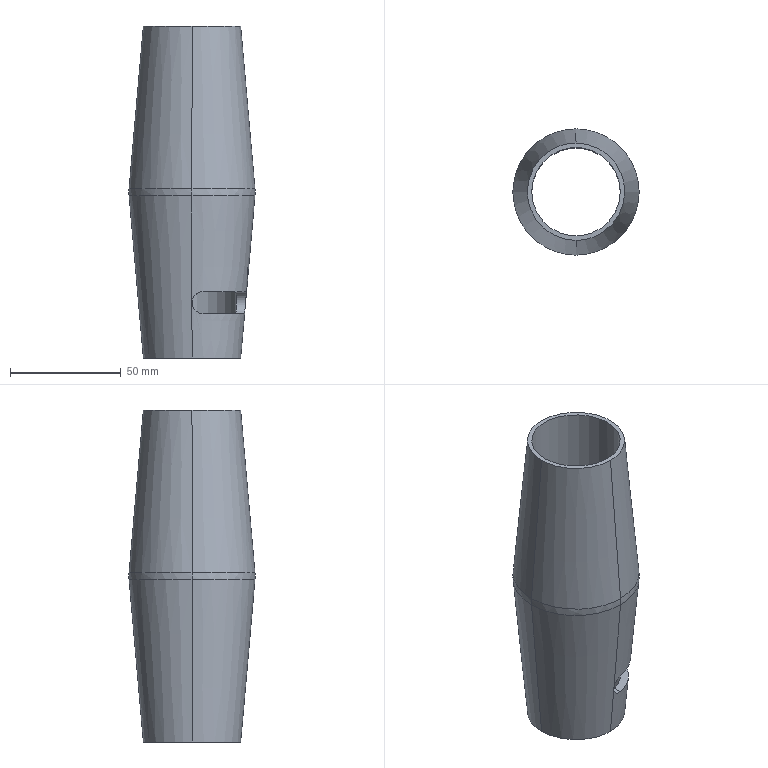Part | NX | features EXTRACT_STRING 12, THRU_CURVE_MESH 8, DATUM_CSYS 6, SKETCH 5, LINE 4, Instance Feature 3, Mirror Feature 3, DATUM_PLANE 2, EXTRACT_DATUM_AXIS 2, EXTRACT_DATUM_PLANE 2, EXTRUDE 2, FILL_HOLE 2, BLEND 1, FACE_BLEND 1, SEW 1 | 1 solid | 20 faces | box 57.039 x 57.039 x 150 mm | volume 113335 mm3 | spline 13 | plane 4 | cylinder 3 | commonest cylinder face diameters 10 x2 40 x1
STEP:
#1=CARTESIAN_POINT('',(28.442,0.000000001,76.752));
#2=VERTEX_POINT('',#1);
#3=CARTESIAN_POINT('',(28.442,0.000000001,73.248));
#4=VERTEX_POINT('',#3);
#5=CARTESIAN_POINT('',(8.519,0.000000001,75.));
#6=DIRECTION('',(0.,1.,0.));
#7=DIRECTION('',(0.,0.,1.));
#8=AXIS2_PLACEMENT_3D('',#5,#6,#7);
#9=CIRCLE('',#8,20.);
#10=EDGE_CURVE('',#2,#4,#9,.T.);
#11=ORIENTED_EDGE('',*,*,#10,.F.);
#12=CARTESIAN_POINT('',(0.,-28.442,76.752));
#13=VERTEX_POINT('',#12);
#14=CARTESIAN_POINT('',(0.,-28.442,76.752));
#15=CARTESIAN_POINT('',(3.703,-28.442,76.752));
#16=CARTESIAN_POINT('',(11.179,-26.96,76.752));
#17=CARTESIAN_POINT('',(20.625,-20.641,76.752));
#18=CARTESIAN_POINT('',(26.948,-11.192,76.752));
#19=CARTESIAN_POINT('',(28.442,-3.756,76.752));
#20=CARTESIAN_POINT('',(28.442,0.000000001,76.752));
#21=B_SPLINE_CURVE_WITH_KNOTS('',3,(#14,#15,#16,#17,#18,#19,#20),.UNSPECIFIED.,.F.,.F.,(4,1,1,1,4),(-0.00000006,0.01111,0.02222,0.03332,0.04443),.UNSPECIFIED.);
#22=EDGE_CURVE('',#13,#2,#21,.T.);
#23=ORIENTED_EDGE('',*,*,#22,.F.);
#24=CARTESIAN_POINT('',(0.,-28.442,73.248));
#25=VERTEX_POINT('',#24);
#26=CARTESIAN_POINT('',(0.,-8.519,75.));
#27=DIRECTION('',(1.,0.,0.));
#28=DIRECTION('',(0.,1.,0.));
#29=AXIS2_PLACEMENT_3D('',#26,#27,#28);
#30=CIRCLE('',#29,20.);
#31=EDGE_CURVE('',#13,#25,#30,.T.);
#32=ORIENTED_EDGE('',*,*,#31,.T.);
#33=CARTESIAN_POINT('',(28.442,0.000000001,73.248));
#34=CARTESIAN_POINT('',(28.442,-3.733,73.248));
#35=CARTESIAN_POINT('',(26.948,-11.202,73.248));
#36=CARTESIAN_POINT('',(20.623,-20.639,73.248));
#37=CARTESIAN_POINT('',(12.759,-25.903,73.248));
#38=CARTESIAN_POINT('',(5.563,-28.078,73.248));
#39=CARTESIAN_POINT('',(1.878,-28.442,73.248));
#40=CARTESIAN_POINT('',(0.,-28.442,73.248));
#41=B_SPLINE_CURVE_WITH_KNOTS('',3,(#33,#34,#35,#36,#37,#38,#39,#40),.UNSPECIFIED.,.F.,.F.,(4,1,1,1,1,4),(-0.00000006,0.0112,0.0224,0.0336,0.03919,0.04479),.UNSPECIFIED.);
#42=EDGE_CURVE('',#4,#25,#41,.T.);
#43=ORIENTED_EDGE('',*,*,#42,.F.);
#44=EDGE_LOOP('',(#11,#23,#32,#43));
#45=FACE_BOUND('',#44,.T.);
#46=CARTESIAN_POINT('',(0.000000001,-28.442,73.248));
#47=CARTESIAN_POINT('',(0.,-28.597,75.));
#48=CARTESIAN_POINT('',(0.,-28.442,76.752));
#49=CARTESIAN_POINT('',(1.895,-28.442,73.248));
#50=CARTESIAN_POINT('',(1.905,-28.597,75.));
#51=CARTESIAN_POINT('',(1.895,-28.442,76.752));
#52=CARTESIAN_POINT('',(5.564,-28.077,73.248));
#53=CARTESIAN_POINT('',(5.594,-28.229,75.));
#54=CARTESIAN_POINT('',(5.564,-28.077,76.752));
#55=CARTESIAN_POINT('',(12.78,-25.896,73.248));
#56=CARTESIAN_POINT('',(12.849,-26.037,75.));
#57=CARTESIAN_POINT('',(12.78,-25.896,76.752));
#58=CARTESIAN_POINT('',(20.647,-20.616,73.248));
#59=CARTESIAN_POINT('',(20.759,-20.728,75.));
#60=CARTESIAN_POINT('',(20.647,-20.616,76.752));
#61=CARTESIAN_POINT('',(25.914,-12.739,73.248));
#62=CARTESIAN_POINT('',(26.054,-12.808,75.));
#63=CARTESIAN_POINT('',(25.914,-12.739,76.752));
#64=CARTESIAN_POINT('',(28.083,-5.538,73.248));
#65=CARTESIAN_POINT('',(28.236,-5.568,75.));
#66=CARTESIAN_POINT('',(28.083,-5.538,76.752));
#67=CARTESIAN_POINT('',(28.442,-1.857,73.248));
#68=CARTESIAN_POINT('',(28.597,-1.867,75.));
#69=CARTESIAN_POINT('',(28.442,-1.857,76.752));
#70=CARTESIAN_POINT('',(28.442,0.000000001,73.248));
#71=CARTESIAN_POINT('',(28.597,0.000000001,75.));
#72=CARTESIAN_POINT('',(28.442,0.000000001,76.752));
#73=(BOUNDED_SURFACE()B_SPLINE_SURFACE(3,2,((#46,#47,#48),(#49,#50,#51),(#52,#53,#54),(#55,#56,#57),(#58,#59,#60),(#61,#62,#63),(#64,#65,#66),(#67,#68,#69),(#70,#71,#72)),.UNSPECIFIED.,.F.,.F.,.F.)B_SPLINE_SURFACE_WITH_KNOTS((4,1,1,1,1,1,4),(3,3),(0.07773,0.07942,0.08111,0.08449,0.08787,0.08956,0.09125),(0.,1.),.UNSPECIFIED.)GEOMETRIC_REPRESENTATION_ITEM()RATIONAL_B_SPLINE_SURFACE(((1.,0.9962,1.),(1.,0.9962,1.),(1.,0.9962,1.),(1.,0.9962,1.),(1.,0.9962,1.),(1.,0.9962,1.),(1.,0.9962,1.),(1.,0.9962,1.),(1.,0.9962,1.)))REPRESENTATION_ITEM('')SURFACE());
#74=ADVANCED_FACE('',(#45),#73,.T.);
#75=ORIENTED_EDGE('',*,*,#31,.F.);
#76=CARTESIAN_POINT('',(-28.442,-0.000000001,76.752));
#77=VERTEX_POINT('',#76);
#78=CARTESIAN_POINT('',(-28.442,0.,76.752));
#79=CARTESIAN_POINT('',(-28.442,-3.733,76.752));
#80=CARTESIAN_POINT('',(-26.948,-11.202,76.752));
#81=CARTESIAN_POINT('',(-20.623,-20.639,76.752));
#82=CARTESIAN_POINT('',(-12.759,-25.903,76.752));
#83=CARTESIAN_POINT('',(-5.563,-28.078,76.752));
#84=CARTESIAN_POINT('',(-1.878,-28.442,76.752));
#85=CARTESIAN_POINT('',(0.,-28.442,76.752));
#86=B_SPLINE_CURVE_WITH_KNOTS('',3,(#78,#79,#80,#81,#82,#83,#84,#85),.UNSPECIFIED.,.F.,.F.,(4,1,1,1,1,4),(-0.00000006,0.0112,0.0224,0.0336,0.03919,0.04479),.UNSPECIFIED.);
#87=EDGE_CURVE('',#77,#13,#86,.T.);
#88=ORIENTED_EDGE('',*,*,#87,.F.);
#89=CARTESIAN_POINT('',(-28.442,0.,73.248));
#90=VERTEX_POINT('',#89);
#91=CARTESIAN_POINT('',(-8.519,0.,75.));
#92=DIRECTION('',(0.,-1.,0.));
#93=DIRECTION('',(0.,0.,-1.));
#94=AXIS2_PLACEMENT_3D('',#91,#92,#93);
#95=CIRCLE('',#94,20.);
#96=EDGE_CURVE('',#77,#90,#95,.T.);
#97=ORIENTED_EDGE('',*,*,#96,.T.);
#98=CARTESIAN_POINT('',(0.,-28.442,73.248));
#99=CARTESIAN_POINT('',(-3.703,-28.442,73.248));
#100=CARTESIAN_POINT('',(-11.179,-26.96,73.248));
#101=CARTESIAN_POINT('',(-20.625,-20.641,73.248));
#102=CARTESIAN_POINT('',(-26.948,-11.192,73.248));
#103=CARTESIAN_POINT('',(-28.442,-3.756,73.248));
#104=CARTESIAN_POINT('',(-28.442,0.,73.248));
#105=B_SPLINE_CURVE_WITH_KNOTS('',3,(#98,#99,#100,#101,#102,#103,#104),.UNSPECIFIED.,.F.,.F.,(4,1,1,1,4),(-0.00000006,0.01111,0.02222,0.03332,0.04443),.UNSPECIFIED.);
#106=EDGE_CURVE('',#25,#90,#105,.T.);
#107=ORIENTED_EDGE('',*,*,#106,.F.);
#108=EDGE_LOOP('',(#75,#88,#97,#107));
#109=FACE_BOUND('',#108,.T.);
#110=CARTESIAN_POINT('',(0.,-28.442,76.752));
#111=CARTESIAN_POINT('',(0.,-28.597,75.));
#112=CARTESIAN_POINT('',(0.,-28.442,73.248));
#113=CARTESIAN_POINT('',(-1.895,-28.442,76.752));
#114=CARTESIAN_POINT('',(-1.905,-28.597,75.));
#115=CARTESIAN_POINT('',(-1.895,-28.442,73.248));
#116=CARTESIAN_POINT('',(-5.564,-28.077,76.752));
#117=CARTESIAN_POINT('',(-5.594,-28.229,75.));
#118=CARTESIAN_POINT('',(-5.564,-28.077,73.248));
#119=CARTESIAN_POINT('',(-12.78,-25.896,76.752));
#120=CARTESIAN_POINT('',(-12.849,-26.037,75.));
#121=CARTESIAN_POINT('',(-12.78,-25.896,73.248));
#122=CARTESIAN_POINT('',(-20.647,-20.616,76.752));
#123=CARTESIAN_POINT('',(-20.759,-20.728,75.));
#124=CARTESIAN_POINT('',(-20.647,-20.616,73.248));
#125=CARTESIAN_POINT('',(-25.914,-12.739,76.752));
#126=CARTESIAN_POINT('',(-26.054,-12.808,75.));
#127=CARTESIAN_POINT('',(-25.914,-12.739,73.248));
#128=CARTESIAN_POINT('',(-28.083,-5.538,76.752));
#129=CARTESIAN_POINT('',(-28.236,-5.568,75.));
#130=CARTESIAN_POINT('',(-28.083,-5.538,73.248));
#131=CARTESIAN_POINT('',(-28.442,-1.857,76.752));
#132=CARTESIAN_POINT('',(-28.597,-1.867,75.));
#133=CARTESIAN_POINT('',(-28.442,-1.857,73.248));
#134=CARTESIAN_POINT('',(-28.442,0.,76.752));
#135=CARTESIAN_POINT('',(-28.597,0.,75.));
#136=CARTESIAN_POINT('',(-28.442,0.,73.248));
#137=(BOUNDED_SURFACE()B_SPLINE_SURFACE(3,2,((#110,#111,#112),(#113,#114,#115),(#116,#117,#118),(#119,#120,#121),(#122,#123,#124),(#125,#126,#127),(#128,#129,#130),(#131,#132,#133),(#134,#135,#136)),.UNSPECIFIED.,.F.,.F.,.F.)B_SPLINE_SURFACE_WITH_KNOTS((4,1,1,1,1,1,4),(3,3),(0.,0.001666,0.003332,0.006664,0.009996,0.01166,0.01333),(0.,1.),.UNSPECIFIED.)GEOMETRIC_REPRESENTATION_ITEM()RATIONAL_B_SPLINE_SURFACE(((1.,0.9962,1.),(1.,0.9962,1.),(1.,0.9962,1.),(1.,0.9962,1.),(1.,0.9962,1.),(1.,0.9962,1.),(1.,0.9962,1.),(1.,0.9962,1.),(1.,0.9962,1.)))REPRESENTATION_ITEM('')SURFACE());
#138=ADVANCED_FACE('',(#109),#137,.T.);
#139=ORIENTED_EDGE('',*,*,#96,.F.);
#140=CARTESIAN_POINT('',(-0.000000001,28.442,76.752));
#141=VERTEX_POINT('',#140);
#142=CARTESIAN_POINT('',(-0.000000001,28.442,76.752));
#143=CARTESIAN_POINT('',(-3.733,28.442,76.752));
#144=CARTESIAN_POINT('',(-11.202,26.948,76.752));
#145=CARTESIAN_POINT('',(-20.639,20.623,76.752));
#146=CARTESIAN_POINT('',(-25.903,12.759,76.752));
#147=CARTESIAN_POINT('',(-28.078,5.563,76.752));
#148=CARTESIAN_POINT('',(-28.442,1.878,76.752));
#149=CARTESIAN_POINT('',(-28.442,-0.000000001,76.752));
#150=B_SPLINE_CURVE_WITH_KNOTS('',3,(#142,#143,#144,#145,#146,#147,#148,#149),.UNSPECIFIED.,.F.,.F.,(4,1,1,1,1,4),(-0.00000006,0.0112,0.0224,0.0336,0.03919,0.04479),.UNSPECIFIED.);
#151=EDGE_CURVE('',#141,#77,#150,.T.);
#152=ORIENTED_EDGE('',*,*,#151,.F.);
#153=CARTESIAN_POINT('',(0.,28.442,73.248));
#154=VERTEX_POINT('',#153);
#155=CARTESIAN_POINT('',(0.,8.519,75.));
#156=DIRECTION('',(-1.,0.,0.));
#157=DIRECTION('',(0.,0.,1.));
#158=AXIS2_PLACEMENT_3D('',#155,#156,#157);
#159=CIRCLE('',#158,20.);
#160=EDGE_CURVE('',#141,#154,#159,.T.);
#161=ORIENTED_EDGE('',*,*,#160,.T.);
#162=CARTESIAN_POINT('',(-28.442,0.,73.248));
#163=CARTESIAN_POINT('',(-28.442,3.703,73.248));
#164=CARTESIAN_POINT('',(-26.96,11.179,73.248));
#165=CARTESIAN_POINT('',(-20.641,20.625,73.248));
#166=CARTESIAN_POINT('',(-11.192,26.948,73.248));
#167=CARTESIAN_POINT('',(-3.756,28.442,73.248));
#168=CARTESIAN_POINT('',(0.,28.442,73.248));
#169=B_SPLINE_CURVE_WITH_KNOTS('',3,(#162,#163,#164,#165,#166,#167,#168),.UNSPECIFIED.,.F.,.F.,(4,1,1,1,4),(-0.00000006,0.01111,0.02222,0.03332,0.04443),.UNSPECIFIED.);
#170=EDGE_CURVE('',#90,#154,#169,.T.);
#171=ORIENTED_EDGE('',*,*,#170,.F.);
#172=EDGE_LOOP('',(#139,#152,#161,#171));
#173=FACE_BOUND('',#172,.T.);
#174=CARTESIAN_POINT('',(-28.442,-0.000000001,76.752));
#175=CARTESIAN_POINT('',(-28.597,0.,75.));
#176=CARTESIAN_POINT('',(-28.442,0.,73.248));
#177=CARTESIAN_POINT('',(-28.442,1.895,76.752));
#178=CARTESIAN_POINT('',(-28.597,1.905,75.));
#179=CARTESIAN_POINT('',(-28.442,1.895,73.248));
#180=CARTESIAN_POINT('',(-28.077,5.564,76.752));
#181=CARTESIAN_POINT('',(-28.229,5.594,75.));
#182=CARTESIAN_POINT('',(-28.077,5.564,73.248));
#183=CARTESIAN_POINT('',(-25.896,12.78,76.752));
#184=CARTESIAN_POINT('',(-26.037,12.849,75.));
#185=CARTESIAN_POINT('',(-25.896,12.78,73.248));
#186=CARTESIAN_POINT('',(-20.616,20.647,76.752));
#187=CARTESIAN_POINT('',(-20.728,20.759,75.));
#188=CARTESIAN_POINT('',(-20.616,20.647,73.248));
#189=CARTESIAN_POINT('',(-12.739,25.914,76.752));
#190=CARTESIAN_POINT('',(-12.808,26.054,75.));
#191=CARTESIAN_POINT('',(-12.739,25.914,73.248));
#192=CARTESIAN_POINT('',(-5.538,28.083,76.752));
#193=CARTESIAN_POINT('',(-5.568,28.236,75.));
#194=CARTESIAN_POINT('',(-5.538,28.083,73.248));
#195=CARTESIAN_POINT('',(-1.857,28.442,76.752));
#196=CARTESIAN_POINT('',(-1.867,28.597,75.));
#197=CARTESIAN_POINT('',(-1.857,28.442,73.248));
#198=CARTESIAN_POINT('',(-0.000000001,28.442,76.752));
#199=CARTESIAN_POINT('',(0.,28.597,75.));
#200=CARTESIAN_POINT('',(0.,28.442,73.248));
#201=(BOUNDED_SURFACE()B_SPLINE_SURFACE(3,2,((#174,#175,#176),(#177,#178,#179),(#180,#181,#182),(#183,#184,#185),(#186,#187,#188),(#189,#190,#191),(#192,#193,#194),(#195,#196,#197),(#198,#199,#200)),.UNSPECIFIED.,.F.,.F.,.F.)B_SPLINE_SURFACE_WITH_KNOTS((4,1,1,1,1,1,4),(3,3),(0.,0.001666,0.003332,0.006664,0.009996,0.01166,0.01333),(0.,1.),.UNSPECIFIED.)GEOMETRIC_REPRESENTATION_ITEM()RATIONAL_B_SPLINE_SURFACE(((1.,0.9962,1.),(1.,0.9962,1.),(1.,0.9962,1.),(1.,0.9962,1.),(1.,0.9962,1.),(1.,0.9962,1.),(1.,0.9962,1.),(1.,0.9962,1.),(1.,0.9962,1.)))REPRESENTATION_ITEM('')SURFACE());
#202=ADVANCED_FACE('',(#173),#201,.T.);
#203=CARTESIAN_POINT('',(28.442,0.000000001,76.752));
#204=CARTESIAN_POINT('',(28.442,3.733,76.752));
#205=CARTESIAN_POINT('',(26.948,11.202,76.752));
#206=CARTESIAN_POINT('',(20.623,20.639,76.752));
#207=CARTESIAN_POINT('',(12.759,25.903,76.752));
#208=CARTESIAN_POINT('',(5.563,28.078,76.752));
#209=CARTESIAN_POINT('',(1.878,28.442,76.752));
#210=CARTESIAN_POINT('',(-0.000000001,28.442,76.752));
#211=B_SPLINE_CURVE_WITH_KNOTS('',3,(#203,#204,#205,#206,#207,#208,#209,#210),.UNSPECIFIED.,.F.,.F.,(4,1,1,1,1,4),(-0.00000006,0.0112,0.0224,0.0336,0.03919,0.04479),.UNSPECIFIED.);
#212=EDGE_CURVE('',#2,#141,#211,.T.);
#213=ORIENTED_EDGE('',*,*,#212,.F.);
#214=ORIENTED_EDGE('',*,*,#10,.T.);
#215=CARTESIAN_POINT('',(-0.000000001,28.442,73.248));
#216=CARTESIAN_POINT('',(3.703,28.442,73.248));
#217=CARTESIAN_POINT('',(11.179,26.96,73.248));
#218=CARTESIAN_POINT('',(20.625,20.641,73.248));
#219=CARTESIAN_POINT('',(26.948,11.192,73.248));
#220=CARTESIAN_POINT('',(28.442,3.756,73.248));
#221=CARTESIAN_POINT('',(28.442,0.000000001,73.248));
#222=B_SPLINE_CURVE_WITH_KNOTS('',3,(#215,#216,#217,#218,#219,#220,#221),.UNSPECIFIED.,.F.,.F.,(4,1,1,1,4),(-0.00000006,0.01111,0.02222,0.03332,0.04443),.UNSPECIFIED.);
#223=EDGE_CURVE('',#154,#4,#222,.T.);
#224=ORIENTED_EDGE('',*,*,#223,.F.);
#225=ORIENTED_EDGE('',*,*,#160,.F.);
#226=EDGE_LOOP('',(#213,#214,#224,#225));
#227=FACE_BOUND('',#226,.T.);
#228=CARTESIAN_POINT('',(-0.000000001,28.442,76.752));
#229=CARTESIAN_POINT('',(-0.000000001,28.597,75.));
#230=CARTESIAN_POINT('',(-0.000000001,28.442,73.248));
#231=CARTESIAN_POINT('',(1.895,28.442,76.752));
#232=CARTESIAN_POINT('',(1.905,28.597,75.));
#233=CARTESIAN_POINT('',(1.895,28.442,73.248));
#234=CARTESIAN_POINT('',(5.564,28.077,76.752));
#235=CARTESIAN_POINT('',(5.594,28.229,75.));
#236=CARTESIAN_POINT('',(5.564,28.077,73.248));
#237=CARTESIAN_POINT('',(12.78,25.896,76.752));
#238=CARTESIAN_POINT('',(12.849,26.037,75.));
#239=CARTESIAN_POINT('',(12.78,25.896,73.248));
#240=CARTESIAN_POINT('',(20.647,20.616,76.752));
#241=CARTESIAN_POINT('',(20.759,20.728,75.));
#242=CARTESIAN_POINT('',(20.647,20.616,73.248));
#243=CARTESIAN_POINT('',(25.914,12.739,76.752));
#244=CARTESIAN_POINT('',(26.054,12.808,75.));
#245=CARTESIAN_POINT('',(25.914,12.739,73.248));
#246=CARTESIAN_POINT('',(28.083,5.538,76.752));
#247=CARTESIAN_POINT('',(28.236,5.568,75.));
#248=CARTESIAN_POINT('',(28.083,5.538,73.248));
#249=CARTESIAN_POINT('',(28.442,1.857,76.752));
#250=CARTESIAN_POINT('',(28.597,1.867,75.));
#251=CARTESIAN_POINT('',(28.442,1.857,73.248));
#252=CARTESIAN_POINT('',(28.442,0.000000001,76.752));
#253=CARTESIAN_POINT('',(28.597,0.000000001,75.));
#254=CARTESIAN_POINT('',(28.442,0.000000001,73.248));
#255=(BOUNDED_SURFACE()B_SPLINE_SURFACE(3,2,((#228,#229,#230),(#231,#232,#233),(#234,#235,#236),(#237,#238,#239),(#240,#241,#242),(#243,#244,#245),(#246,#247,#248),(#249,#250,#251),(#252,#253,#254)),.UNSPECIFIED.,.F.,.F.,.F.)B_SPLINE_SURFACE_WITH_KNOTS((4,1,1,1,1,1,4),(3,3),(0.,0.001666,0.003332,0.006664,0.009996,0.01166,0.01333),(0.,1.),.UNSPECIFIED.)GEOMETRIC_REPRESENTATION_ITEM()RATIONAL_B_SPLINE_SURFACE(((1.,0.9962,1.),(1.,0.9962,1.),(1.,0.9962,1.),(1.,0.9962,1.),(1.,0.9962,1.),(1.,0.9962,1.),(1.,0.9962,1.),(1.,0.9962,1.),(1.,0.9962,1.)))REPRESENTATION_ITEM('')SURFACE());
#256=ADVANCED_FACE('',(#227),#255,.T.);
#257=CARTESIAN_POINT('',(24.199,0.,25.));
#258=VERTEX_POINT('',#257);
#259=CARTESIAN_POINT('',(28.597,0.000000001,75.));
#260=CARTESIAN_POINT('',(26.398,0.000000001,50.));
#261=CARTESIAN_POINT('',(24.199,0.,25.));
#262=CARTESIAN_POINT('',(22.,0.,0.));
#263=B_SPLINE_CURVE_WITH_KNOTS('',3,(#259,#260,#261,#262),.UNSPECIFIED.,.F.,.F.,(4,4),(0.,1.),.PIECEWISE_BEZIER_KNOTS.);
#264=EDGE_CURVE('',#258,#4,#263,.F.);
#265=ORIENTED_EDGE('',*,*,#264,.T.);
#266=ORIENTED_EDGE('',*,*,#42,.T.);
#267=CARTESIAN_POINT('',(0.,-24.199,25.));
#268=VERTEX_POINT('',#267);
#269=CARTESIAN_POINT('',(0.,-28.597,75.));
#270=CARTESIAN_POINT('',(0.,-26.398,50.));
#271=CARTESIAN_POINT('',(0.,-24.199,25.));
#272=CARTESIAN_POINT('',(0.,-22.,0.));
#273=B_SPLINE_CURVE_WITH_KNOTS('',3,(#269,#270,#271,#272),.UNSPECIFIED.,.F.,.F.,(4,4),(0.,1.),.PIECEWISE_BEZIER_KNOTS.);
#274=EDGE_CURVE('',#25,#268,#273,.T.);
#275=ORIENTED_EDGE('',*,*,#274,.T.);
#276=CARTESIAN_POINT('',(5.,-24.126,30.));
#277=VERTEX_POINT('',#276);
#278=CARTESIAN_POINT('',(0.,-24.199,25.));
#279=CARTESIAN_POINT('',(0.,-24.315,26.321));
#280=CARTESIAN_POINT('',(1.085,-24.577,28.918));
#281=CARTESIAN_POINT('',(3.701,-24.395,30.));
#282=CARTESIAN_POINT('',(5.,-24.126,30.));
#283=B_SPLINE_CURVE_WITH_KNOTS('',3,(#278,#279,#280,#281,#282),.UNSPECIFIED.,.F.,.F.,(4,1,4),(0.,0.003922,0.007844),.UNSPECIFIED.);
#284=EDGE_CURVE('',#268,#277,#283,.T.);
#285=ORIENTED_EDGE('',*,*,#284,.T.);
#286=CARTESIAN_POINT('',(24.126,-5.,30.));
#287=VERTEX_POINT('',#286);
#288=CARTESIAN_POINT('',(24.126,-5.,30.));
#289=CARTESIAN_POINT('',(23.162,-9.652,30.));
#290=CARTESIAN_POINT('',(18.401,-18.452,30.));
#291=CARTESIAN_POINT('',(9.708,-23.15,30.));
#292=CARTESIAN_POINT('',(5.,-24.126,30.));
#293=B_SPLINE_CURVE_WITH_KNOTS('',3,(#288,#289,#290,#291,#292),.UNSPECIFIED.,.F.,.F.,(4,1,4),(0.005015,0.01926,0.0335),.UNSPECIFIED.);
#294=EDGE_CURVE('',#287,#277,#293,.T.);
#295=ORIENTED_EDGE('',*,*,#294,.F.);
#296=CARTESIAN_POINT('',(24.126,-5.,30.));
#297=CARTESIAN_POINT('',(24.395,-3.702,30.));
#298=CARTESIAN_POINT('',(24.577,-1.09,28.923));
#299=CARTESIAN_POINT('',(24.315,0.,26.321));
#300=CARTESIAN_POINT('',(24.199,0.,25.));
#301=B_SPLINE_CURVE_WITH_KNOTS('',3,(#296,#297,#298,#299,#300),.UNSPECIFIED.,.F.,.F.,(4,1,4),(0.,0.003923,0.007845),.UNSPECIFIED.);
#302=EDGE_CURVE('',#287,#258,#301,.T.);
#303=ORIENTED_EDGE('',*,*,#302,.T.);
#304=EDGE_LOOP('',(#265,#266,#275,#285,#295,#303));
#305=FACE_BOUND('',#304,.T.);
#306=CARTESIAN_POINT('',(28.468,0.000000001,73.537));
#307=CARTESIAN_POINT('',(28.468,-1.863,73.537));
#308=CARTESIAN_POINT('',(28.101,-5.59,73.537));
#309=CARTESIAN_POINT('',(26.47,-10.964,73.537));
#310=CARTESIAN_POINT('',(23.823,-15.918,73.537));
#311=CARTESIAN_POINT('',(20.26,-20.26,73.537));
#312=CARTESIAN_POINT('',(15.918,-23.823,73.537));
#313=CARTESIAN_POINT('',(10.964,-26.47,73.537));
#314=CARTESIAN_POINT('',(5.59,-28.101,73.537));
#315=CARTESIAN_POINT('',(1.863,-28.468,73.537));
#316=CARTESIAN_POINT('',(0.000000001,-28.468,73.537));
#317=CARTESIAN_POINT('',(27.036,0.000000001,57.262));
#318=CARTESIAN_POINT('',(27.036,-1.77,57.262));
#319=CARTESIAN_POINT('',(26.688,-5.309,57.262));
#320=CARTESIAN_POINT('',(25.139,-10.413,57.262));
#321=CARTESIAN_POINT('',(22.625,-15.117,57.262));
#322=CARTESIAN_POINT('',(19.241,-19.241,57.262));
#323=CARTESIAN_POINT('',(15.117,-22.625,57.262));
#324=CARTESIAN_POINT('',(10.413,-25.139,57.262));
#325=CARTESIAN_POINT('',(5.309,-26.688,57.262));
#326=CARTESIAN_POINT('',(1.77,-27.036,57.262));
#327=CARTESIAN_POINT('',(0.000000001,-27.036,57.262));
#328=CARTESIAN_POINT('',(25.605,0.000000001,40.986));
#329=CARTESIAN_POINT('',(25.605,-1.676,40.986));
#330=CARTESIAN_POINT('',(25.275,-5.027,40.986));
#331=CARTESIAN_POINT('',(23.808,-9.862,40.986));
#332=CARTESIAN_POINT('',(21.427,-14.317,40.986));
#333=CARTESIAN_POINT('',(18.222,-18.222,40.986));
#334=CARTESIAN_POINT('',(14.317,-21.427,40.986));
#335=CARTESIAN_POINT('',(9.862,-23.808,40.986));
#336=CARTESIAN_POINT('',(5.027,-25.275,40.986));
#337=CARTESIAN_POINT('',(1.676,-25.605,40.986));
#338=CARTESIAN_POINT('',(0.000000001,-25.605,40.986));
#339=CARTESIAN_POINT('',(24.173,0.,24.711));
#340=CARTESIAN_POINT('',(24.173,-1.582,24.711));
#341=CARTESIAN_POINT('',(23.862,-4.746,24.711));
#342=CARTESIAN_POINT('',(22.477,-9.31,24.711));
#343=CARTESIAN_POINT('',(20.229,-13.517,24.711));
#344=CARTESIAN_POINT('',(17.203,-17.203,24.711));
#345=CARTESIAN_POINT('',(13.517,-20.229,24.711));
#346=CARTESIAN_POINT('',(9.31,-22.477,24.711));
#347=CARTESIAN_POINT('',(4.746,-23.862,24.711));
#348=CARTESIAN_POINT('',(1.582,-24.173,24.711));
#349=CARTESIAN_POINT('',(0.,-24.173,24.711));
#350=B_SPLINE_SURFACE_WITH_KNOTS('',3,3,((#306,#307,#308,#309,#310,#311,#312,#313,#314,#315,#316),(#317,#318,#319,#320,#321,#322,#323,#324,#325,#326,#327),(#328,#329,#330,#331,#332,#333,#334,#335,#336,#337,#338),(#339,#340,#341,#342,#343,#344,#345,#346,#347,#348,#349)),.RULED_SURF.,.F.,.F.,.F.,(4,4),(4,1,1,1,1,1,1,1,4),(0.0195,0.6705),(0.,0.125,0.25,0.375,0.5,0.625,0.75,0.875,1.),.UNSPECIFIED.);
#351=ADVANCED_FACE('',(#305),#350,.F.);
#352=CARTESIAN_POINT('',(20.,0.,150.));
#353=VERTEX_POINT('',#352);
#354=CARTESIAN_POINT('',(0.,0.,150.));
#355=DIRECTION('',(0.,0.,1.));
#356=DIRECTION('',(1.,0.,0.));
#357=AXIS2_PLACEMENT_3D('',#354,#355,#356);
#358=CIRCLE('',#357,20.);
#359=EDGE_CURVE('',#353,#353,#358,.F.);
#360=ORIENTED_EDGE('',*,*,#359,.F.);
#361=EDGE_LOOP('',(#360));
#362=FACE_BOUND('',#361,.T.);
#363=CARTESIAN_POINT('',(20.,0.,0.));
#364=VERTEX_POINT('',#363);
#365=CARTESIAN_POINT('',(0.,0.,0.));
#366=DIRECTION('',(0.,0.,1.));
#367=DIRECTION('',(1.,0.,0.));
#368=AXIS2_PLACEMENT_3D('',#365,#366,#367);
#369=CIRCLE('',#368,20.);
#370=EDGE_CURVE('',#364,#364,#369,.T.);
#371=ORIENTED_EDGE('',*,*,#370,.F.);
#372=EDGE_LOOP('',(#371));
#373=FACE_BOUND('',#372,.T.);
#374=CARTESIAN_POINT('',(19.365,-5.,20.));
#375=VERTEX_POINT('',#374);
#376=CARTESIAN_POINT('',(19.365,-5.,30.));
#377=VERTEX_POINT('',#376);
#378=CARTESIAN_POINT('',(19.365,-5.,20.));
#379=CARTESIAN_POINT('',(19.697,-3.713,20.));
#380=CARTESIAN_POINT('',(20.041,-1.109,21.049));
#381=CARTESIAN_POINT('',(19.979,0.5536,25.002));
#382=CARTESIAN_POINT('',(20.042,-1.105,28.945));
#383=CARTESIAN_POINT('',(19.697,-3.713,30.));
#384=CARTESIAN_POINT('',(19.365,-5.,30.));
#385=B_SPLINE_CURVE_WITH_KNOTS('',3,(#378,#379,#380,#381,#382,#383,#384),.UNSPECIFIED.,.F.,.F.,(4,1,1,1,4),(0.,0.003931,0.007862,0.01179,0.01572),.UNSPECIFIED.);
#386=EDGE_CURVE('',#375,#377,#385,.T.);
#387=ORIENTED_EDGE('',*,*,#386,.T.);
#388=CARTESIAN_POINT('',(5.,-19.365,30.));
#389=VERTEX_POINT('',#388);
#390=CARTESIAN_POINT('',(0.,0.,30.));
#391=DIRECTION('',(0.,0.,-1.));
#392=DIRECTION('',(-1.,0.,0.));
#393=AXIS2_PLACEMENT_3D('',#390,#391,#392);
#394=CIRCLE('',#393,20.);
#395=EDGE_CURVE('',#377,#389,#394,.T.);
#396=ORIENTED_EDGE('',*,*,#395,.T.);
#397=CARTESIAN_POINT('',(5.,-19.365,20.));
#398=VERTEX_POINT('',#397);
#399=CARTESIAN_POINT('',(5.,-19.365,30.));
#400=CARTESIAN_POINT('',(3.713,-19.697,30.));
#401=CARTESIAN_POINT('',(1.109,-20.041,28.951));
#402=CARTESIAN_POINT('',(-0.5536,-19.979,24.998));
#403=CARTESIAN_POINT('',(1.105,-20.042,21.055));
#404=CARTESIAN_POINT('',(3.713,-19.697,20.));
#405=CARTESIAN_POINT('',(5.,-19.365,20.));
#406=B_SPLINE_CURVE_WITH_KNOTS('',3,(#399,#400,#401,#402,#403,#404,#405),.UNSPECIFIED.,.F.,.F.,(4,1,1,1,4),(0.,0.003931,0.007862,0.01179,0.01572),.UNSPECIFIED.);
#407=EDGE_CURVE('',#389,#398,#406,.T.);
#408=ORIENTED_EDGE('',*,*,#407,.T.);
#409=CARTESIAN_POINT('',(0.,0.,20.));
#410=DIRECTION('',(0.,0.,-1.));
#411=DIRECTION('',(-1.,0.,0.));
#412=AXIS2_PLACEMENT_3D('',#409,#410,#411);
#413=CIRCLE('',#412,20.);
#414=EDGE_CURVE('',#375,#398,#413,.T.);
#415=ORIENTED_EDGE('',*,*,#414,.F.);
#416=EDGE_LOOP('',(#387,#396,#408,#415));
#417=FACE_BOUND('',#416,.T.);
#418=CARTESIAN_POINT('',(0.,0.,177.));
#419=DIRECTION('',(0.,0.,-1.));
#420=DIRECTION('',(-1.,0.,0.));
#421=AXIS2_PLACEMENT_3D('',#418,#419,#420);
#422=CYLINDRICAL_SURFACE('',#421,20.);
#423=ADVANCED_FACE('',(#362,#373,#417),#422,.F.);
#424=CARTESIAN_POINT('',(0.,22.,150.));
#425=VERTEX_POINT('',#424);
#426=CARTESIAN_POINT('',(0.,22.,150.));
#427=CARTESIAN_POINT('',(0.,24.199,125.));
#428=CARTESIAN_POINT('',(0.,26.398,100.));
#429=CARTESIAN_POINT('',(-0.000000001,28.597,75.));
#430=B_SPLINE_CURVE_WITH_KNOTS('',3,(#426,#427,#428,#429),.UNSPECIFIED.,.F.,.F.,(4,4),(0.,1.),.PIECEWISE_BEZIER_KNOTS.);
#431=EDGE_CURVE('',#141,#425,#430,.F.);
#432=ORIENTED_EDGE('',*,*,#431,.F.);
#433=ORIENTED_EDGE('',*,*,#151,.T.);
#434=CARTESIAN_POINT('',(-22.,0.,150.));
#435=VERTEX_POINT('',#434);
#436=CARTESIAN_POINT('',(-22.,0.,150.));
#437=CARTESIAN_POINT('',(-24.199,0.,125.));
#438=CARTESIAN_POINT('',(-26.398,0.,100.));
#439=CARTESIAN_POINT('',(-28.597,-0.000000001,75.));
#440=B_SPLINE_CURVE_WITH_KNOTS('',3,(#436,#437,#438,#439),.UNSPECIFIED.,.F.,.F.,(4,4),(0.,1.),.PIECEWISE_BEZIER_KNOTS.);
#441=EDGE_CURVE('',#435,#77,#440,.T.);
#442=ORIENTED_EDGE('',*,*,#441,.F.);
#443=CARTESIAN_POINT('',(-22.,0.,150.));
#444=CARTESIAN_POINT('',(-22.,5.758,150.));
#445=CARTESIAN_POINT('',(-17.232,17.234,150.));
#446=CARTESIAN_POINT('',(-5.761,22.,150.));
#447=CARTESIAN_POINT('',(0.,22.,150.));
#448=B_SPLINE_CURVE_WITH_KNOTS('',3,(#443,#444,#445,#446,#447),.UNSPECIFIED.,.F.,.F.,(4,1,4),(0.,0.5,1.),.UNSPECIFIED.);
#449=EDGE_CURVE('',#425,#435,#448,.F.);
#450=ORIENTED_EDGE('',*,*,#449,.F.);
#451=EDGE_LOOP('',(#432,#433,#442,#450));
#452=FACE_BOUND('',#451,.T.);
#453=CARTESIAN_POINT('',(-22.,0.,150.));
#454=CARTESIAN_POINT('',(-22.,1.44,150.));
#455=CARTESIAN_POINT('',(-21.716,4.32,150.));
#456=CARTESIAN_POINT('',(-20.456,8.473,150.));
#457=CARTESIAN_POINT('',(-18.41,12.301,150.));
#458=CARTESIAN_POINT('',(-15.657,15.657,150.));
#459=CARTESIAN_POINT('',(-12.301,18.41,150.));
#460=CARTESIAN_POINT('',(-8.473,20.456,150.));
#461=CARTESIAN_POINT('',(-4.32,21.716,150.));
#462=CARTESIAN_POINT('',(-1.44,22.,150.));
#463=CARTESIAN_POINT('',(0.,22.,150.));
#464=CARTESIAN_POINT('',(-24.16,0.,125.438));
#465=CARTESIAN_POINT('',(-24.16,1.581,125.438));
#466=CARTESIAN_POINT('',(-23.849,4.744,125.438));
#467=CARTESIAN_POINT('',(-22.465,9.305,125.438));
#468=CARTESIAN_POINT('',(-20.218,13.509,125.438));
#469=CARTESIAN_POINT('',(-17.194,17.194,125.438));
#470=CARTESIAN_POINT('',(-13.509,20.218,125.438));
#471=CARTESIAN_POINT('',(-9.305,22.465,125.438));
#472=CARTESIAN_POINT('',(-4.744,23.849,125.438));
#473=CARTESIAN_POINT('',(-1.581,24.16,125.438));
#474=CARTESIAN_POINT('',(0.,24.16,125.438));
#475=CARTESIAN_POINT('',(-26.321,0.,100.875));
#476=CARTESIAN_POINT('',(-26.321,1.723,100.875));
#477=CARTESIAN_POINT('',(-25.981,5.168,100.875));
#478=CARTESIAN_POINT('',(-24.474,10.137,100.875));
#479=CARTESIAN_POINT('',(-22.026,14.717,100.875));
#480=CARTESIAN_POINT('',(-18.732,18.732,100.875));
#481=CARTESIAN_POINT('',(-14.717,22.026,100.875));
#482=CARTESIAN_POINT('',(-10.137,24.474,100.875));
#483=CARTESIAN_POINT('',(-5.168,25.981,100.875));
#484=CARTESIAN_POINT('',(-1.723,26.321,100.875));
#485=CARTESIAN_POINT('',(0.,26.321,100.875));
#486=CARTESIAN_POINT('',(-28.481,-0.000000001,76.313));
#487=CARTESIAN_POINT('',(-28.481,1.864,76.313));
#488=CARTESIAN_POINT('',(-28.114,5.592,76.313));
#489=CARTESIAN_POINT('',(-26.483,10.97,76.313));
#490=CARTESIAN_POINT('',(-23.834,15.925,76.313));
#491=CARTESIAN_POINT('',(-20.269,20.269,76.313));
#492=CARTESIAN_POINT('',(-15.925,23.834,76.313));
#493=CARTESIAN_POINT('',(-10.97,26.483,76.313));
#494=CARTESIAN_POINT('',(-5.592,28.114,76.313));
#495=CARTESIAN_POINT('',(-1.864,28.481,76.313));
#496=CARTESIAN_POINT('',(-0.000000001,28.481,76.313));
#497=B_SPLINE_SURFACE_WITH_KNOTS('',3,3,((#453,#454,#455,#456,#457,#458,#459,#460,#461,#462,#463),(#464,#465,#466,#467,#468,#469,#470,#471,#472,#473,#474),(#475,#476,#477,#478,#479,#480,#481,#482,#483,#484,#485),(#486,#487,#488,#489,#490,#491,#492,#493,#494,#495,#496)),.RULED_SURF.,.F.,.F.,.F.,(4,4),(4,1,1,1,1,1,1,1,4),(0.,0.9825),(0.,0.125,0.25,0.375,0.5,0.625,0.75,0.875,1.),.UNSPECIFIED.);
#498=ADVANCED_FACE('',(#452),#497,.F.);
#499=ORIENTED_EDGE('',*,*,#441,.T.);
#500=ORIENTED_EDGE('',*,*,#87,.T.);
#501=CARTESIAN_POINT('',(0.,-22.,150.));
#502=VERTEX_POINT('',#501);
#503=CARTESIAN_POINT('',(0.,-22.,150.));
#504=CARTESIAN_POINT('',(0.,-24.199,125.));
#505=CARTESIAN_POINT('',(0.,-26.398,100.));
#506=CARTESIAN_POINT('',(0.,-28.597,75.));
#507=B_SPLINE_CURVE_WITH_KNOTS('',3,(#503,#504,#505,#506),.UNSPECIFIED.,.F.,.F.,(4,4),(0.,1.),.PIECEWISE_BEZIER_KNOTS.);
#508=EDGE_CURVE('',#13,#502,#507,.F.);
#509=ORIENTED_EDGE('',*,*,#508,.T.);
#510=CARTESIAN_POINT('',(0.,-22.,150.));
#511=CARTESIAN_POINT('',(-5.758,-22.,150.));
#512=CARTESIAN_POINT('',(-17.234,-17.232,150.));
#513=CARTESIAN_POINT('',(-22.,-5.761,150.));
#514=CARTESIAN_POINT('',(-22.,0.,150.));
#515=B_SPLINE_CURVE_WITH_KNOTS('',3,(#510,#511,#512,#513,#514),.UNSPECIFIED.,.F.,.F.,(4,1,4),(0.,0.5,1.),.UNSPECIFIED.);
#516=EDGE_CURVE('',#502,#435,#515,.T.);
#517=ORIENTED_EDGE('',*,*,#516,.T.);
#518=EDGE_LOOP('',(#499,#500,#509,#517));
#519=FACE_BOUND('',#518,.T.);
#520=CARTESIAN_POINT('',(-22.,0.,150.));
#521=CARTESIAN_POINT('',(-22.,-1.44,150.));
#522=CARTESIAN_POINT('',(-21.716,-4.32,150.));
#523=CARTESIAN_POINT('',(-20.456,-8.473,150.));
#524=CARTESIAN_POINT('',(-18.41,-12.301,150.));
#525=CARTESIAN_POINT('',(-15.657,-15.657,150.));
#526=CARTESIAN_POINT('',(-12.301,-18.41,150.));
#527=CARTESIAN_POINT('',(-8.473,-20.456,150.));
#528=CARTESIAN_POINT('',(-4.32,-21.716,150.));
#529=CARTESIAN_POINT('',(-1.44,-22.,150.));
#530=CARTESIAN_POINT('',(0.,-22.,150.));
#531=CARTESIAN_POINT('',(-24.16,0.,125.438));
#532=CARTESIAN_POINT('',(-24.16,-1.581,125.438));
#533=CARTESIAN_POINT('',(-23.849,-4.744,125.438));
#534=CARTESIAN_POINT('',(-22.465,-9.305,125.438));
#535=CARTESIAN_POINT('',(-20.218,-13.509,125.438));
#536=CARTESIAN_POINT('',(-17.194,-17.194,125.438));
#537=CARTESIAN_POINT('',(-13.509,-20.218,125.438));
#538=CARTESIAN_POINT('',(-9.305,-22.465,125.438));
#539=CARTESIAN_POINT('',(-4.744,-23.849,125.438));
#540=CARTESIAN_POINT('',(-1.581,-24.16,125.438));
#541=CARTESIAN_POINT('',(0.,-24.16,125.438));
#542=CARTESIAN_POINT('',(-26.321,0.,100.875));
#543=CARTESIAN_POINT('',(-26.321,-1.723,100.875));
#544=CARTESIAN_POINT('',(-25.981,-5.168,100.875));
#545=CARTESIAN_POINT('',(-24.474,-10.137,100.875));
#546=CARTESIAN_POINT('',(-22.026,-14.717,100.875));
#547=CARTESIAN_POINT('',(-18.732,-18.732,100.875));
#548=CARTESIAN_POINT('',(-14.717,-22.026,100.875));
#549=CARTESIAN_POINT('',(-10.137,-24.474,100.875));
#550=CARTESIAN_POINT('',(-5.168,-25.981,100.875));
#551=CARTESIAN_POINT('',(-1.723,-26.321,100.875));
#552=CARTESIAN_POINT('',(0.,-26.321,100.875));
#553=CARTESIAN_POINT('',(-28.481,0.,76.313));
#554=CARTESIAN_POINT('',(-28.481,-1.864,76.313));
#555=CARTESIAN_POINT('',(-28.114,-5.592,76.313));
#556=CARTESIAN_POINT('',(-26.483,-10.97,76.313));
#557=CARTESIAN_POINT('',(-23.834,-15.925,76.313));
#558=CARTESIAN_POINT('',(-20.269,-20.269,76.313));
#559=CARTESIAN_POINT('',(-15.925,-23.834,76.313));
#560=CARTESIAN_POINT('',(-10.97,-26.483,76.313));
#561=CARTESIAN_POINT('',(-5.592,-28.114,76.313));
#562=CARTESIAN_POINT('',(-1.864,-28.481,76.313));
#563=CARTESIAN_POINT('',(0.,-28.481,76.313));
#564=B_SPLINE_SURFACE_WITH_KNOTS('',3,3,((#520,#521,#522,#523,#524,#525,#526,#527,#528,#529,#530),(#531,#532,#533,#534,#535,#536,#537,#538,#539,#540,#541),(#542,#543,#544,#545,#546,#547,#548,#549,#550,#551,#552),(#553,#554,#555,#556,#557,#558,#559,#560,#561,#562,#563)),.RULED_SURF.,.F.,.F.,.F.,(4,4),(4,1,1,1,1,1,1,1,4),(0.,0.9825),(0.,0.125,0.25,0.375,0.5,0.625,0.75,0.875,1.),.UNSPECIFIED.);
#565=ADVANCED_FACE('',(#519),#564,.T.);
#566=CARTESIAN_POINT('',(-22.,0.,0.));
#567=VERTEX_POINT('',#566);
#568=CARTESIAN_POINT('',(-28.597,0.,75.));
#569=CARTESIAN_POINT('',(-26.398,0.,50.));
#570=CARTESIAN_POINT('',(-24.199,0.,25.));
#571=CARTESIAN_POINT('',(-22.,0.,0.));
#572=B_SPLINE_CURVE_WITH_KNOTS('',3,(#568,#569,#570,#571),.UNSPECIFIED.,.F.,.F.,(4,4),(0.,1.),.PIECEWISE_BEZIER_KNOTS.);
#573=EDGE_CURVE('',#90,#567,#572,.T.);
#574=ORIENTED_EDGE('',*,*,#573,.F.);
#575=ORIENTED_EDGE('',*,*,#170,.T.);
#576=CARTESIAN_POINT('',(0.,22.,0.));
#577=VERTEX_POINT('',#576);
#578=CARTESIAN_POINT('',(0.,28.597,75.));
#579=CARTESIAN_POINT('',(0.,26.398,50.));
#580=CARTESIAN_POINT('',(0.,24.199,25.));
#581=CARTESIAN_POINT('',(0.,22.,0.));
#582=B_SPLINE_CURVE_WITH_KNOTS('',3,(#578,#579,#580,#581),.UNSPECIFIED.,.F.,.F.,(4,4),(0.,1.),.PIECEWISE_BEZIER_KNOTS.);
#583=EDGE_CURVE('',#577,#154,#582,.F.);
#584=ORIENTED_EDGE('',*,*,#583,.F.);
#585=CARTESIAN_POINT('',(0.,22.,0.));
#586=CARTESIAN_POINT('',(-5.758,22.,0.));
#587=CARTESIAN_POINT('',(-17.234,17.232,0.));
#588=CARTESIAN_POINT('',(-22.,5.761,0.));
#589=CARTESIAN_POINT('',(-22.,0.,0.));
#590=B_SPLINE_CURVE_WITH_KNOTS('',3,(#585,#586,#587,#588,#589),.UNSPECIFIED.,.F.,.F.,(4,1,4),(0.,0.5,1.),.UNSPECIFIED.);
#591=EDGE_CURVE('',#567,#577,#590,.F.);
#592=ORIENTED_EDGE('',*,*,#591,.F.);
#593=EDGE_LOOP('',(#574,#575,#584,#592));
#594=FACE_BOUND('',#593,.T.);
#595=CARTESIAN_POINT('',(-28.481,0.,73.687));
#596=CARTESIAN_POINT('',(-28.481,1.864,73.687));
#597=CARTESIAN_POINT('',(-28.114,5.592,73.687));
#598=CARTESIAN_POINT('',(-26.483,10.97,73.687));
#599=CARTESIAN_POINT('',(-23.834,15.925,73.687));
#600=CARTESIAN_POINT('',(-20.269,20.269,73.687));
#601=CARTESIAN_POINT('',(-15.925,23.834,73.687));
#602=CARTESIAN_POINT('',(-10.97,26.483,73.687));
#603=CARTESIAN_POINT('',(-5.592,28.114,73.687));
#604=CARTESIAN_POINT('',(-1.864,28.481,73.687));
#605=CARTESIAN_POINT('',(0.,28.481,73.687));
#606=CARTESIAN_POINT('',(-26.321,0.,49.125));
#607=CARTESIAN_POINT('',(-26.321,1.723,49.125));
#608=CARTESIAN_POINT('',(-25.981,5.168,49.125));
#609=CARTESIAN_POINT('',(-24.474,10.137,49.125));
#610=CARTESIAN_POINT('',(-22.026,14.717,49.125));
#611=CARTESIAN_POINT('',(-18.732,18.732,49.125));
#612=CARTESIAN_POINT('',(-14.717,22.026,49.125));
#613=CARTESIAN_POINT('',(-10.137,24.474,49.125));
#614=CARTESIAN_POINT('',(-5.168,25.981,49.125));
#615=CARTESIAN_POINT('',(-1.723,26.321,49.125));
#616=CARTESIAN_POINT('',(0.,26.321,49.125));
#617=CARTESIAN_POINT('',(-24.16,0.,24.562));
#618=CARTESIAN_POINT('',(-24.16,1.581,24.562));
#619=CARTESIAN_POINT('',(-23.849,4.744,24.562));
#620=CARTESIAN_POINT('',(-22.465,9.305,24.562));
#621=CARTESIAN_POINT('',(-20.218,13.509,24.562));
#622=CARTESIAN_POINT('',(-17.194,17.194,24.562));
#623=CARTESIAN_POINT('',(-13.509,20.218,24.562));
#624=CARTESIAN_POINT('',(-9.305,22.465,24.562));
#625=CARTESIAN_POINT('',(-4.744,23.849,24.562));
#626=CARTESIAN_POINT('',(-1.581,24.16,24.562));
#627=CARTESIAN_POINT('',(0.,24.16,24.562));
#628=CARTESIAN_POINT('',(-22.,0.,0.));
#629=CARTESIAN_POINT('',(-22.,1.44,0.));
#630=CARTESIAN_POINT('',(-21.716,4.32,0.));
#631=CARTESIAN_POINT('',(-20.456,8.473,0.));
#632=CARTESIAN_POINT('',(-18.41,12.301,0.));
#633=CARTESIAN_POINT('',(-15.657,15.657,0.));
#634=CARTESIAN_POINT('',(-12.301,18.41,0.));
#635=CARTESIAN_POINT('',(-8.473,20.456,0.));
#636=CARTESIAN_POINT('',(-4.32,21.716,0.));
#637=CARTESIAN_POINT('',(-1.44,22.,0.));
#638=CARTESIAN_POINT('',(0.,22.,0.));
#639=B_SPLINE_SURFACE_WITH_KNOTS('',3,3,((#595,#596,#597,#598,#599,#600,#601,#602,#603,#604,#605),(#606,#607,#608,#609,#610,#611,#612,#613,#614,#615,#616),(#617,#618,#619,#620,#621,#622,#623,#624,#625,#626,#627),(#628,#629,#630,#631,#632,#633,#634,#635,#636,#637,#638)),.RULED_SURF.,.F.,.F.,.F.,(4,4),(4,1,1,1,1,1,1,1,4),(0.0175,1.),(0.,0.125,0.25,0.375,0.5,0.625,0.75,0.875,1.),.UNSPECIFIED.);
#640=ADVANCED_FACE('',(#594),#639,.F.);
#641=CARTESIAN_POINT('',(22.,0.,150.));
#642=VERTEX_POINT('',#641);
#643=CARTESIAN_POINT('',(22.,0.,150.));
#644=CARTESIAN_POINT('',(24.199,0.,125.));
#645=CARTESIAN_POINT('',(26.398,0.,100.));
#646=CARTESIAN_POINT('',(28.597,0.000000001,75.));
#647=B_SPLINE_CURVE_WITH_KNOTS('',3,(#643,#644,#645,#646),.UNSPECIFIED.,.F.,.F.,(4,4),(0.,1.),.PIECEWISE_BEZIER_KNOTS.);
#648=EDGE_CURVE('',#2,#642,#647,.F.);
#649=ORIENTED_EDGE('',*,*,#648,.F.);
#650=ORIENTED_EDGE('',*,*,#212,.T.);
#651=ORIENTED_EDGE('',*,*,#431,.T.);
#652=CARTESIAN_POINT('',(0.,22.,150.));
#653=CARTESIAN_POINT('',(5.758,22.,150.));
#654=CARTESIAN_POINT('',(17.234,17.232,150.));
#655=CARTESIAN_POINT('',(22.,5.761,150.));
#656=CARTESIAN_POINT('',(22.,0.,150.));
#657=B_SPLINE_CURVE_WITH_KNOTS('',3,(#652,#653,#654,#655,#656),.UNSPECIFIED.,.F.,.F.,(4,1,4),(0.,0.5,1.),.UNSPECIFIED.);
#658=EDGE_CURVE('',#642,#425,#657,.F.);
#659=ORIENTED_EDGE('',*,*,#658,.F.);
#660=EDGE_LOOP('',(#649,#650,#651,#659));
#661=FACE_BOUND('',#660,.T.);
#662=CARTESIAN_POINT('',(0.,22.,150.));
#663=CARTESIAN_POINT('',(1.44,22.,150.));
#664=CARTESIAN_POINT('',(4.32,21.716,150.));
#665=CARTESIAN_POINT('',(8.473,20.456,150.));
#666=CARTESIAN_POINT('',(12.301,18.41,150.));
#667=CARTESIAN_POINT('',(15.657,15.657,150.));
#668=CARTESIAN_POINT('',(18.41,12.301,150.));
#669=CARTESIAN_POINT('',(20.456,8.473,150.));
#670=CARTESIAN_POINT('',(21.716,4.32,150.));
#671=CARTESIAN_POINT('',(22.,1.44,150.));
#672=CARTESIAN_POINT('',(22.,0.,150.));
#673=CARTESIAN_POINT('',(0.,24.16,125.438));
#674=CARTESIAN_POINT('',(1.581,24.16,125.438));
#675=CARTESIAN_POINT('',(4.744,23.849,125.438));
#676=CARTESIAN_POINT('',(9.305,22.465,125.438));
#677=CARTESIAN_POINT('',(13.509,20.218,125.438));
#678=CARTESIAN_POINT('',(17.194,17.194,125.438));
#679=CARTESIAN_POINT('',(20.218,13.509,125.438));
#680=CARTESIAN_POINT('',(22.465,9.305,125.438));
#681=CARTESIAN_POINT('',(23.849,4.744,125.438));
#682=CARTESIAN_POINT('',(24.16,1.581,125.438));
#683=CARTESIAN_POINT('',(24.16,0.,125.438));
#684=CARTESIAN_POINT('',(0.,26.321,100.875));
#685=CARTESIAN_POINT('',(1.723,26.321,100.875));
#686=CARTESIAN_POINT('',(5.168,25.981,100.875));
#687=CARTESIAN_POINT('',(10.137,24.474,100.875));
#688=CARTESIAN_POINT('',(14.717,22.026,100.875));
#689=CARTESIAN_POINT('',(18.732,18.732,100.875));
#690=CARTESIAN_POINT('',(22.026,14.717,100.875));
#691=CARTESIAN_POINT('',(24.474,10.137,100.875));
#692=CARTESIAN_POINT('',(25.981,5.168,100.875));
#693=CARTESIAN_POINT('',(26.321,1.723,100.875));
#694=CARTESIAN_POINT('',(26.321,0.,100.875));
#695=CARTESIAN_POINT('',(-0.000000001,28.481,76.313));
#696=CARTESIAN_POINT('',(1.864,28.481,76.313));
#697=CARTESIAN_POINT('',(5.592,28.114,76.313));
#698=CARTESIAN_POINT('',(10.97,26.483,76.313));
#699=CARTESIAN_POINT('',(15.925,23.834,76.313));
#700=CARTESIAN_POINT('',(20.269,20.269,76.313));
#701=CARTESIAN_POINT('',(23.834,15.925,76.313));
#702=CARTESIAN_POINT('',(26.483,10.97,76.313));
#703=CARTESIAN_POINT('',(28.114,5.592,76.313));
#704=CARTESIAN_POINT('',(28.481,1.864,76.313));
#705=CARTESIAN_POINT('',(28.481,0.000000001,76.313));
#706=B_SPLINE_SURFACE_WITH_KNOTS('',3,3,((#662,#663,#664,#665,#666,#667,#668,#669,#670,#671,#672),(#673,#674,#675,#676,#677,#678,#679,#680,#681,#682,#683),(#684,#685,#686,#687,#688,#689,#690,#691,#692,#693,#694),(#695,#696,#697,#698,#699,#700,#701,#702,#703,#704,#705)),.RULED_SURF.,.F.,.F.,.F.,(4,4),(4,1,1,1,1,1,1,1,4),(0.,0.9825),(0.,0.125,0.25,0.375,0.5,0.625,0.75,0.875,1.),.UNSPECIFIED.);
#707=ADVANCED_FACE('',(#661),#706,.F.);
#708=ORIENTED_EDGE('',*,*,#359,.T.);
#709=EDGE_LOOP('',(#708));
#710=FACE_BOUND('',#709,.T.);
#711=CARTESIAN_POINT('',(22.,0.,150.));
#712=CARTESIAN_POINT('',(22.,-5.763,150.));
#713=CARTESIAN_POINT('',(17.23,-17.231,150.));
#714=CARTESIAN_POINT('',(5.766,-22.,150.));
#715=CARTESIAN_POINT('',(0.,-22.,150.));
#716=B_SPLINE_CURVE_WITH_KNOTS('',3,(#711,#712,#713,#714,#715),.UNSPECIFIED.,.F.,.F.,(4,1,4),(0.,0.5,1.),.UNSPECIFIED.);
#717=EDGE_CURVE('',#642,#502,#716,.T.);
#718=ORIENTED_EDGE('',*,*,#717,.F.);
#719=ORIENTED_EDGE('',*,*,#658,.T.);
#720=ORIENTED_EDGE('',*,*,#449,.T.);
#721=ORIENTED_EDGE('',*,*,#516,.F.);
#722=EDGE_LOOP('',(#718,#719,#720,#721));
#723=FACE_BOUND('',#722,.T.);
#724=CARTESIAN_POINT('',(0.,0.,150.));
#725=DIRECTION('',(0.,0.,1.));
#726=DIRECTION('',(1.,0.,0.));
#727=AXIS2_PLACEMENT_3D('',#724,#725,#726);
#728=PLANE('',#727);
#729=ADVANCED_FACE('',(#710,#723),#728,.T.);
#730=ORIENTED_EDGE('',*,*,#274,.F.);
#731=ORIENTED_EDGE('',*,*,#106,.T.);
#732=ORIENTED_EDGE('',*,*,#573,.T.);
#733=CARTESIAN_POINT('',(0.,-22.,0.));
#734=VERTEX_POINT('',#733);
#735=CARTESIAN_POINT('',(-22.,0.,0.));
#736=CARTESIAN_POINT('',(-22.,-5.758,0.));
#737=CARTESIAN_POINT('',(-17.232,-17.234,0.));
#738=CARTESIAN_POINT('',(-5.761,-22.,0.));
#739=CARTESIAN_POINT('',(0.,-22.,0.));
#740=B_SPLINE_CURVE_WITH_KNOTS('',3,(#735,#736,#737,#738,#739),.UNSPECIFIED.,.F.,.F.,(4,1,4),(0.,0.5,1.),.UNSPECIFIED.);
#741=EDGE_CURVE('',#734,#567,#740,.F.);
#742=ORIENTED_EDGE('',*,*,#741,.F.);
#743=CARTESIAN_POINT('',(0.,-28.597,75.));
#744=CARTESIAN_POINT('',(0.,-26.398,50.));
#745=CARTESIAN_POINT('',(0.,-24.199,25.));
#746=CARTESIAN_POINT('',(0.,-22.,0.));
#747=B_SPLINE_CURVE_WITH_KNOTS('',3,(#743,#744,#745,#746),.UNSPECIFIED.,.F.,.F.,(4,4),(0.,1.),.PIECEWISE_BEZIER_KNOTS.);
#748=EDGE_CURVE('',#268,#734,#747,.T.);
#749=ORIENTED_EDGE('',*,*,#748,.F.);
#750=EDGE_LOOP('',(#730,#731,#732,#742,#749));
#751=FACE_BOUND('',#750,.T.);
#752=CARTESIAN_POINT('',(-28.481,0.,73.687));
#753=CARTESIAN_POINT('',(-26.321,0.,49.125));
#754=CARTESIAN_POINT('',(-24.16,0.,24.562));
#755=CARTESIAN_POINT('',(-22.,0.,0.));
#756=CARTESIAN_POINT('',(-28.481,-1.864,73.687));
#757=CARTESIAN_POINT('',(-26.321,-1.723,49.125));
#758=CARTESIAN_POINT('',(-24.16,-1.581,24.562));
#759=CARTESIAN_POINT('',(-22.,-1.44,0.));
#760=CARTESIAN_POINT('',(-28.114,-5.592,73.687));
#761=CARTESIAN_POINT('',(-25.981,-5.168,49.125));
#762=CARTESIAN_POINT('',(-23.849,-4.744,24.562));
#763=CARTESIAN_POINT('',(-21.716,-4.32,0.));
#764=CARTESIAN_POINT('',(-26.483,-10.97,73.687));
#765=CARTESIAN_POINT('',(-24.474,-10.137,49.125));
#766=CARTESIAN_POINT('',(-22.465,-9.305,24.562));
#767=CARTESIAN_POINT('',(-20.456,-8.473,0.));
#768=CARTESIAN_POINT('',(-23.834,-15.925,73.687));
#769=CARTESIAN_POINT('',(-22.026,-14.717,49.125));
#770=CARTESIAN_POINT('',(-20.218,-13.509,24.562));
#771=CARTESIAN_POINT('',(-18.41,-12.301,0.));
#772=CARTESIAN_POINT('',(-20.269,-20.269,73.687));
#773=CARTESIAN_POINT('',(-18.732,-18.732,49.125));
#774=CARTESIAN_POINT('',(-17.194,-17.194,24.562));
#775=CARTESIAN_POINT('',(-15.657,-15.657,0.));
#776=CARTESIAN_POINT('',(-15.925,-23.834,73.687));
#777=CARTESIAN_POINT('',(-14.717,-22.026,49.125));
#778=CARTESIAN_POINT('',(-13.509,-20.218,24.562));
#779=CARTESIAN_POINT('',(-12.301,-18.41,0.));
#780=CARTESIAN_POINT('',(-10.97,-26.483,73.687));
#781=CARTESIAN_POINT('',(-10.137,-24.474,49.125));
#782=CARTESIAN_POINT('',(-9.305,-22.465,24.562));
#783=CARTESIAN_POINT('',(-8.473,-20.456,0.));
#784=CARTESIAN_POINT('',(-5.592,-28.114,73.687));
#785=CARTESIAN_POINT('',(-5.168,-25.981,49.125));
#786=CARTESIAN_POINT('',(-4.744,-23.849,24.562));
#787=CARTESIAN_POINT('',(-4.32,-21.716,0.));
#788=CARTESIAN_POINT('',(-1.864,-28.481,73.687));
#789=CARTESIAN_POINT('',(-1.723,-26.321,49.125));
#790=CARTESIAN_POINT('',(-1.581,-24.16,24.562));
#791=CARTESIAN_POINT('',(-1.44,-22.,0.));
#792=CARTESIAN_POINT('',(0.,-28.481,73.687));
#793=CARTESIAN_POINT('',(0.,-26.321,49.125));
#794=CARTESIAN_POINT('',(0.,-24.16,24.562));
#795=CARTESIAN_POINT('',(0.,-22.,0.));
#796=B_SPLINE_SURFACE_WITH_KNOTS('',3,3,((#752,#753,#754,#755),(#756,#757,#758,#759),(#760,#761,#762,#763),(#764,#765,#766,#767),(#768,#769,#770,#771),(#772,#773,#774,#775),(#776,#777,#778,#779),(#780,#781,#782,#783),(#784,#785,#786,#787),(#788,#789,#790,#791),(#792,#793,#794,#795)),.RULED_SURF.,.F.,.F.,.F.,(4,1,1,1,1,1,1,1,4),(4,4),(0.,0.125,0.25,0.375,0.5,0.625,0.75,0.875,1.),(0.0175,1.),.UNSPECIFIED.);
#797=ADVANCED_FACE('',(#751),#796,.F.);
#798=ORIENTED_EDGE('',*,*,#508,.F.);
#799=ORIENTED_EDGE('',*,*,#22,.T.);
#800=ORIENTED_EDGE('',*,*,#648,.T.);
#801=ORIENTED_EDGE('',*,*,#717,.T.);
#802=EDGE_LOOP('',(#798,#799,#800,#801));
#803=FACE_BOUND('',#802,.T.);
#804=CARTESIAN_POINT('',(22.,0.,150.));
#805=CARTESIAN_POINT('',(22.,-1.44,150.));
#806=CARTESIAN_POINT('',(21.716,-4.32,150.));
#807=CARTESIAN_POINT('',(20.456,-8.473,150.));
#808=CARTESIAN_POINT('',(18.41,-12.301,150.));
#809=CARTESIAN_POINT('',(15.657,-15.657,150.));
#810=CARTESIAN_POINT('',(12.301,-18.41,150.));
#811=CARTESIAN_POINT('',(8.473,-20.456,150.));
#812=CARTESIAN_POINT('',(4.32,-21.716,150.));
#813=CARTESIAN_POINT('',(1.44,-22.,150.));
#814=CARTESIAN_POINT('',(0.,-22.,150.));
#815=CARTESIAN_POINT('',(24.16,0.,125.438));
#816=CARTESIAN_POINT('',(24.16,-1.581,125.438));
#817=CARTESIAN_POINT('',(23.849,-4.744,125.438));
#818=CARTESIAN_POINT('',(22.465,-9.305,125.438));
#819=CARTESIAN_POINT('',(20.218,-13.509,125.438));
#820=CARTESIAN_POINT('',(17.194,-17.194,125.438));
#821=CARTESIAN_POINT('',(13.509,-20.218,125.438));
#822=CARTESIAN_POINT('',(9.305,-22.465,125.438));
#823=CARTESIAN_POINT('',(4.744,-23.849,125.438));
#824=CARTESIAN_POINT('',(1.581,-24.16,125.438));
#825=CARTESIAN_POINT('',(0.,-24.16,125.438));
#826=CARTESIAN_POINT('',(26.321,0.,100.875));
#827=CARTESIAN_POINT('',(26.321,-1.723,100.875));
#828=CARTESIAN_POINT('',(25.981,-5.168,100.875));
#829=CARTESIAN_POINT('',(24.474,-10.137,100.875));
#830=CARTESIAN_POINT('',(22.026,-14.717,100.875));
#831=CARTESIAN_POINT('',(18.732,-18.732,100.875));
#832=CARTESIAN_POINT('',(14.717,-22.026,100.875));
#833=CARTESIAN_POINT('',(10.137,-24.474,100.875));
#834=CARTESIAN_POINT('',(5.168,-25.981,100.875));
#835=CARTESIAN_POINT('',(1.723,-26.321,100.875));
#836=CARTESIAN_POINT('',(0.,-26.321,100.875));
#837=CARTESIAN_POINT('',(28.481,0.,76.313));
#838=CARTESIAN_POINT('',(28.481,-1.864,76.313));
#839=CARTESIAN_POINT('',(28.114,-5.592,76.313));
#840=CARTESIAN_POINT('',(26.483,-10.97,76.313));
#841=CARTESIAN_POINT('',(23.834,-15.925,76.313));
#842=CARTESIAN_POINT('',(20.269,-20.269,76.313));
#843=CARTESIAN_POINT('',(15.925,-23.834,76.313));
#844=CARTESIAN_POINT('',(10.97,-26.483,76.313));
#845=CARTESIAN_POINT('',(5.592,-28.114,76.313));
#846=CARTESIAN_POINT('',(1.864,-28.481,76.313));
#847=CARTESIAN_POINT('',(0.,-28.481,76.313));
#848=B_SPLINE_SURFACE_WITH_KNOTS('',3,3,((#804,#805,#806,#807,#808,#809,#810,#811,#812,#813,#814),(#815,#816,#817,#818,#819,#820,#821,#822,#823,#824,#825),(#826,#827,#828,#829,#830,#831,#832,#833,#834,#835,#836),(#837,#838,#839,#840,#841,#842,#843,#844,#845,#846,#847)),.RULED_SURF.,.F.,.F.,.F.,(4,4),(4,1,1,1,1,1,1,1,4),(0.,0.9825),(0.,0.125,0.25,0.375,0.5,0.625,0.75,0.875,1.),.UNSPECIFIED.);
#849=ADVANCED_FACE('',(#803),#848,.F.);
#850=ORIENTED_EDGE('',*,*,#370,.T.);
#851=EDGE_LOOP('',(#850));
#852=FACE_BOUND('',#851,.T.);
#853=CARTESIAN_POINT('',(22.,0.,0.));
#854=VERTEX_POINT('',#853);
#855=CARTESIAN_POINT('',(0.,-22.,0.));
#856=CARTESIAN_POINT('',(5.763,-22.,0.));
#857=CARTESIAN_POINT('',(17.231,-17.23,0.));
#858=CARTESIAN_POINT('',(22.,-5.766,0.));
#859=CARTESIAN_POINT('',(22.,0.,0.));
#860=B_SPLINE_CURVE_WITH_KNOTS('',3,(#855,#856,#857,#858,#859),.UNSPECIFIED.,.F.,.F.,(4,1,4),(0.,0.5,1.),.UNSPECIFIED.);
#861=EDGE_CURVE('',#854,#734,#860,.F.);
#862=ORIENTED_EDGE('',*,*,#861,.T.);
#863=ORIENTED_EDGE('',*,*,#741,.T.);
#864=ORIENTED_EDGE('',*,*,#591,.T.);
#865=CARTESIAN_POINT('',(22.,0.,0.));
#866=CARTESIAN_POINT('',(22.,5.763,0.));
#867=CARTESIAN_POINT('',(17.23,17.231,0.));
#868=CARTESIAN_POINT('',(5.766,22.,0.));
#869=CARTESIAN_POINT('',(0.,22.,0.));
#870=B_SPLINE_CURVE_WITH_KNOTS('',3,(#865,#866,#867,#868,#869),.UNSPECIFIED.,.F.,.F.,(4,1,4),(0.,0.5,1.),.UNSPECIFIED.);
#871=EDGE_CURVE('',#577,#854,#870,.F.);
#872=ORIENTED_EDGE('',*,*,#871,.T.);
#873=EDGE_LOOP('',(#862,#863,#864,#872));
#874=FACE_BOUND('',#873,.T.);
#875=CARTESIAN_POINT('',(0.,0.,0.));
#876=DIRECTION('',(0.,0.,1.));
#877=DIRECTION('',(1.,0.,0.));
#878=AXIS2_PLACEMENT_3D('',#875,#876,#877);
#879=PLANE('',#878);
#880=ADVANCED_FACE('',(#852,#874),#879,.F.);
#881=ORIENTED_EDGE('',*,*,#583,.T.);
#882=ORIENTED_EDGE('',*,*,#223,.T.);
#883=ORIENTED_EDGE('',*,*,#264,.F.);
#884=CARTESIAN_POINT('',(28.597,0.000000001,75.));
#885=CARTESIAN_POINT('',(26.398,0.000000001,50.));
#886=CARTESIAN_POINT('',(24.199,0.,25.));
#887=CARTESIAN_POINT('',(22.,0.,0.));
#888=B_SPLINE_CURVE_WITH_KNOTS('',3,(#884,#885,#886,#887),.UNSPECIFIED.,.F.,.F.,(4,4),(0.,1.),.PIECEWISE_BEZIER_KNOTS.);
#889=EDGE_CURVE('',#854,#258,#888,.F.);
#890=ORIENTED_EDGE('',*,*,#889,.F.);
#891=ORIENTED_EDGE('',*,*,#871,.F.);
#892=EDGE_LOOP('',(#881,#882,#883,#890,#891));
#893=FACE_BOUND('',#892,.T.);
#894=CARTESIAN_POINT('',(-0.000000001,28.481,73.687));
#895=CARTESIAN_POINT('',(1.864,28.481,73.687));
#896=CARTESIAN_POINT('',(5.592,28.114,73.687));
#897=CARTESIAN_POINT('',(10.97,26.483,73.687));
#898=CARTESIAN_POINT('',(15.925,23.834,73.687));
#899=CARTESIAN_POINT('',(20.269,20.269,73.687));
#900=CARTESIAN_POINT('',(23.834,15.925,73.687));
#901=CARTESIAN_POINT('',(26.483,10.97,73.687));
#902=CARTESIAN_POINT('',(28.114,5.592,73.687));
#903=CARTESIAN_POINT('',(28.481,1.864,73.687));
#904=CARTESIAN_POINT('',(28.481,0.000000001,73.687));
#905=CARTESIAN_POINT('',(-0.000000001,26.321,49.125));
#906=CARTESIAN_POINT('',(1.723,26.321,49.125));
#907=CARTESIAN_POINT('',(5.168,25.981,49.125));
#908=CARTESIAN_POINT('',(10.137,24.474,49.125));
#909=CARTESIAN_POINT('',(14.717,22.026,49.125));
#910=CARTESIAN_POINT('',(18.732,18.732,49.125));
#911=CARTESIAN_POINT('',(22.026,14.717,49.125));
#912=CARTESIAN_POINT('',(24.474,10.137,49.125));
#913=CARTESIAN_POINT('',(25.981,5.168,49.125));
#914=CARTESIAN_POINT('',(26.321,1.723,49.125));
#915=CARTESIAN_POINT('',(26.321,0.000000001,49.125));
#916=CARTESIAN_POINT('',(0.,24.16,24.562));
#917=CARTESIAN_POINT('',(1.581,24.16,24.562));
#918=CARTESIAN_POINT('',(4.744,23.849,24.562));
#919=CARTESIAN_POINT('',(9.305,22.465,24.562));
#920=CARTESIAN_POINT('',(13.509,20.218,24.562));
#921=CARTESIAN_POINT('',(17.194,17.194,24.562));
#922=CARTESIAN_POINT('',(20.218,13.509,24.562));
#923=CARTESIAN_POINT('',(22.465,9.305,24.562));
#924=CARTESIAN_POINT('',(23.849,4.744,24.562));
#925=CARTESIAN_POINT('',(24.16,1.581,24.562));
#926=CARTESIAN_POINT('',(24.16,0.,24.562));
#927=CARTESIAN_POINT('',(0.,22.,0.));
#928=CARTESIAN_POINT('',(1.44,22.,0.));
#929=CARTESIAN_POINT('',(4.32,21.716,0.));
#930=CARTESIAN_POINT('',(8.473,20.456,0.));
#931=CARTESIAN_POINT('',(12.301,18.41,0.));
#932=CARTESIAN_POINT('',(15.657,15.657,0.));
#933=CARTESIAN_POINT('',(18.41,12.301,0.));
#934=CARTESIAN_POINT('',(20.456,8.473,0.));
#935=CARTESIAN_POINT('',(21.716,4.32,0.));
#936=CARTESIAN_POINT('',(22.,1.44,0.));
#937=CARTESIAN_POINT('',(22.,0.,0.));
#938=B_SPLINE_SURFACE_WITH_KNOTS('',3,3,((#894,#895,#896,#897,#898,#899,#900,#901,#902,#903,#904),(#905,#906,#907,#908,#909,#910,#911,#912,#913,#914,#915),(#916,#917,#918,#919,#920,#921,#922,#923,#924,#925,#926),(#927,#928,#929,#930,#931,#932,#933,#934,#935,#936,#937)),.RULED_SURF.,.F.,.F.,.F.,(4,4),(4,1,1,1,1,1,1,1,4),(0.0175,1.),(0.,0.125,0.25,0.375,0.5,0.625,0.75,0.875,1.),.UNSPECIFIED.);
#939=ADVANCED_FACE('',(#893),#938,.F.);
#940=ORIENTED_EDGE('',*,*,#889,.T.);
#941=CARTESIAN_POINT('',(23.227,-5.,20.));
#942=VERTEX_POINT('',#941);
#943=CARTESIAN_POINT('',(24.199,0.,25.));
#944=CARTESIAN_POINT('',(24.082,0.,23.673));
#945=CARTESIAN_POINT('',(23.888,-1.101,21.071));
#946=CARTESIAN_POINT('',(23.507,-3.698,20.));
#947=CARTESIAN_POINT('',(23.227,-5.,20.));
#948=B_SPLINE_CURVE_WITH_KNOTS('',3,(#943,#944,#945,#946,#947),.UNSPECIFIED.,.F.,.F.,(4,1,4),(0.,0.003938,0.007877),.UNSPECIFIED.);
#949=EDGE_CURVE('',#258,#942,#948,.T.);
#950=ORIENTED_EDGE('',*,*,#949,.T.);
#951=CARTESIAN_POINT('',(5.,-23.227,20.));
#952=VERTEX_POINT('',#951);
#953=CARTESIAN_POINT('',(23.227,-5.,20.));
#954=CARTESIAN_POINT('',(22.275,-9.421,20.));
#955=CARTESIAN_POINT('',(17.715,-17.768,20.));
#956=CARTESIAN_POINT('',(9.476,-22.263,20.));
#957=CARTESIAN_POINT('',(5.,-23.227,20.));
#958=B_SPLINE_CURVE_WITH_KNOTS('',3,(#953,#954,#955,#956,#957),.UNSPECIFIED.,.F.,.F.,(4,1,4),(0.005018,0.01857,0.03213),.UNSPECIFIED.);
#959=EDGE_CURVE('',#942,#952,#958,.T.);
#960=ORIENTED_EDGE('',*,*,#959,.T.);
#961=CARTESIAN_POINT('',(5.,-23.227,20.));
#962=CARTESIAN_POINT('',(3.698,-23.507,20.));
#963=CARTESIAN_POINT('',(1.106,-23.887,21.066));
#964=CARTESIAN_POINT('',(0.,-24.082,23.673));
#965=CARTESIAN_POINT('',(0.,-24.199,25.));
#966=B_SPLINE_CURVE_WITH_KNOTS('',3,(#961,#962,#963,#964,#965),.UNSPECIFIED.,.F.,.F.,(4,1,4),(0.,0.003938,0.007877),.UNSPECIFIED.);
#967=EDGE_CURVE('',#952,#268,#966,.T.);
#968=ORIENTED_EDGE('',*,*,#967,.T.);
#969=ORIENTED_EDGE('',*,*,#748,.T.);
#970=ORIENTED_EDGE('',*,*,#861,.F.);
#971=EDGE_LOOP('',(#940,#950,#960,#968,#969,#970));
#972=FACE_BOUND('',#971,.T.);
#973=CARTESIAN_POINT('',(24.212,0.,25.15));
#974=CARTESIAN_POINT('',(24.212,-1.585,25.15));
#975=CARTESIAN_POINT('',(23.9,-4.754,25.15));
#976=CARTESIAN_POINT('',(22.513,-9.325,25.15));
#977=CARTESIAN_POINT('',(20.261,-13.538,25.15));
#978=CARTESIAN_POINT('',(17.231,-17.231,25.15));
#979=CARTESIAN_POINT('',(13.538,-20.261,25.15));
#980=CARTESIAN_POINT('',(9.325,-22.513,25.15));
#981=CARTESIAN_POINT('',(4.754,-23.9,25.15));
#982=CARTESIAN_POINT('',(1.585,-24.212,25.15));
#983=CARTESIAN_POINT('',(0.,-24.212,25.15));
#984=CARTESIAN_POINT('',(23.475,0.,16.767));
#985=CARTESIAN_POINT('',(23.475,-1.536,16.767));
#986=CARTESIAN_POINT('',(23.172,-4.609,16.767));
#987=CARTESIAN_POINT('',(21.828,-9.041,16.767));
#988=CARTESIAN_POINT('',(19.644,-13.126,16.767));
#989=CARTESIAN_POINT('',(16.706,-16.706,16.767));
#990=CARTESIAN_POINT('',(13.126,-19.644,16.767));
#991=CARTESIAN_POINT('',(9.041,-21.828,16.767));
#992=CARTESIAN_POINT('',(4.609,-23.172,16.767));
#993=CARTESIAN_POINT('',(1.536,-23.475,16.767));
#994=CARTESIAN_POINT('',(0.,-23.475,16.767));
#995=CARTESIAN_POINT('',(22.737,0.,8.383));
#996=CARTESIAN_POINT('',(22.737,-1.488,8.383));
#997=CARTESIAN_POINT('',(22.444,-4.464,8.383));
#998=CARTESIAN_POINT('',(21.142,-8.757,8.383));
#999=CARTESIAN_POINT('',(19.027,-12.714,8.383));
#1000=CARTESIAN_POINT('',(16.181,-16.181,8.383));
#1001=CARTESIAN_POINT('',(12.714,-19.027,8.383));
#1002=CARTESIAN_POINT('',(8.757,-21.142,8.383));
#1003=CARTESIAN_POINT('',(4.464,-22.444,8.383));
#1004=CARTESIAN_POINT('',(1.488,-22.737,8.383));
#1005=CARTESIAN_POINT('',(0.,-22.737,8.383));
#1006=CARTESIAN_POINT('',(22.,0.,0.));
#1007=CARTESIAN_POINT('',(22.,-1.44,0.));
#1008=CARTESIAN_POINT('',(21.716,-4.32,0.));
#1009=CARTESIAN_POINT('',(20.456,-8.473,0.));
#1010=CARTESIAN_POINT('',(18.41,-12.301,0.));
#1011=CARTESIAN_POINT('',(15.657,-15.657,0.));
#1012=CARTESIAN_POINT('',(12.301,-18.41,0.));
#1013=CARTESIAN_POINT('',(8.473,-20.456,0.));
#1014=CARTESIAN_POINT('',(4.32,-21.716,0.));
#1015=CARTESIAN_POINT('',(1.44,-22.,0.));
#1016=CARTESIAN_POINT('',(0.,-22.,0.));
#1017=B_SPLINE_SURFACE_WITH_KNOTS('',3,3,((#973,#974,#975,#976,#977,#978,#979,#980,#981,#982,#983),(#984,#985,#986,#987,#988,#989,#990,#991,#992,#993,#994),(#995,#996,#997,#998,#999,#1000,#1001,#1002,#1003,#1004,#1005),(#1006,#1007,#1008,#1009,#1010,#1011,#1012,#1013,#1014,#1015,#1016)),.RULED_SURF.,.F.,.F.,.F.,(4,4),(4,1,1,1,1,1,1,1,4),(0.6647,1.),(0.,0.125,0.25,0.375,0.5,0.625,0.75,0.875,1.),.UNSPECIFIED.);
#1018=ADVANCED_FACE('',(#972),#1017,.F.);
#1019=ORIENTED_EDGE('',*,*,#294,.T.);
#1020=CARTESIAN_POINT('',(5.,0.,30.));
#1021=DIRECTION('',(0.,-1.,0.));
#1022=VECTOR('',#1021,1000.);
#1023=LINE('',#1020,#1022);
#1024=EDGE_CURVE('',#277,#389,#1023,.F.);
#1025=ORIENTED_EDGE('',*,*,#1024,.T.);
#1026=ORIENTED_EDGE('',*,*,#395,.F.);
#1027=CARTESIAN_POINT('',(0.,-5.,30.));
#1028=DIRECTION('',(-1.,0.,0.));
#1029=VECTOR('',#1028,1000.);
#1030=LINE('',#1027,#1029);
#1031=EDGE_CURVE('',#377,#287,#1030,.F.);
#1032=ORIENTED_EDGE('',*,*,#1031,.T.);
#1033=EDGE_LOOP('',(#1019,#1025,#1026,#1032));
#1034=FACE_BOUND('',#1033,.T.);
#1035=CARTESIAN_POINT('',(0.,0.,30.));
#1036=DIRECTION('',(0.,0.,-1.));
#1037=DIRECTION('',(-1.,0.,0.));
#1038=AXIS2_PLACEMENT_3D('',#1035,#1036,#1037);
#1039=PLANE('',#1038);
#1040=ADVANCED_FACE('',(#1034),#1039,.T.);
#1041=ORIENTED_EDGE('',*,*,#414,.T.);
#1042=CARTESIAN_POINT('',(5.,-23.759,20.));
#1043=DIRECTION('',(0.,-1.,0.));
#1044=VECTOR('',#1043,1000.);
#1045=LINE('',#1042,#1044);
#1046=EDGE_CURVE('',#398,#952,#1045,.T.);
#1047=ORIENTED_EDGE('',*,*,#1046,.T.);
#1048=ORIENTED_EDGE('',*,*,#959,.F.);
#1049=CARTESIAN_POINT('',(20.,-5.,20.));
#1050=DIRECTION('',(-1.,0.,0.));
#1051=VECTOR('',#1050,1000.);
#1052=LINE('',#1049,#1051);
#1053=EDGE_CURVE('',#942,#375,#1052,.T.);
#1054=ORIENTED_EDGE('',*,*,#1053,.T.);
#1055=EDGE_LOOP('',(#1041,#1047,#1048,#1054));
#1056=FACE_BOUND('',#1055,.T.);
#1057=CARTESIAN_POINT('',(0.,0.,20.));
#1058=DIRECTION('',(0.,0.,-1.));
#1059=DIRECTION('',(-1.,0.,0.));
#1060=AXIS2_PLACEMENT_3D('',#1057,#1058,#1059);
#1061=PLANE('',#1060);
#1062=ADVANCED_FACE('',(#1056),#1061,.F.);
#1063=ORIENTED_EDGE('',*,*,#1046,.F.);
#1064=ORIENTED_EDGE('',*,*,#407,.F.);
#1065=ORIENTED_EDGE('',*,*,#1024,.F.);
#1066=ORIENTED_EDGE('',*,*,#284,.F.);
#1067=ORIENTED_EDGE('',*,*,#967,.F.);
#1068=EDGE_LOOP('',(#1063,#1064,#1065,#1066,#1067));
#1069=FACE_BOUND('',#1068,.T.);
#1070=CARTESIAN_POINT('',(5.,0.,25.));
#1071=DIRECTION('',(0.,1.,0.));
#1072=DIRECTION('',(0.,0.,1.));
#1073=AXIS2_PLACEMENT_3D('',#1070,#1071,#1072);
#1074=CYLINDRICAL_SURFACE('',#1073,5.);
#1075=ADVANCED_FACE('',(#1069),#1074,.F.);
#1076=ORIENTED_EDGE('',*,*,#1031,.F.);
#1077=ORIENTED_EDGE('',*,*,#386,.F.);
#1078=ORIENTED_EDGE('',*,*,#1053,.F.);
#1079=ORIENTED_EDGE('',*,*,#949,.F.);
#1080=ORIENTED_EDGE('',*,*,#302,.F.);
#1081=EDGE_LOOP('',(#1076,#1077,#1078,#1079,#1080));
#1082=FACE_BOUND('',#1081,.T.);
#1083=CARTESIAN_POINT('',(0.,-5.,25.));
#1084=DIRECTION('',(-1.,0.,0.));
#1085=DIRECTION('',(0.,0.,1.));
#1086=AXIS2_PLACEMENT_3D('',#1083,#1084,#1085);
#1087=CYLINDRICAL_SURFACE('',#1086,5.);
#1088=ADVANCED_FACE('',(#1082),#1087,.F.);
#1089=CLOSED_SHELL('',(#74,#138,#202,#256,#351,#423,#498,#565,#640,#707,#729,#797,#849,#880,#939,#1018,#1040,#1062,#1075,#1088));
#1090=MANIFOLD_SOLID_BREP('',#1089);
#1091=(LENGTH_UNIT()NAMED_UNIT(*)SI_UNIT(.MILLI.,.METRE.));
#1092=UNCERTAINTY_MEASURE_WITH_UNIT(LENGTH_MEASURE(0.0508),#1091,'','');
#1093=(NAMED_UNIT(*)PLANE_ANGLE_UNIT()SI_UNIT($,.RADIAN.));
#1094=(NAMED_UNIT(*)SI_UNIT($,.STERADIAN.)SOLID_ANGLE_UNIT());
#1095=(GEOMETRIC_REPRESENTATION_CONTEXT(3)GLOBAL_UNCERTAINTY_ASSIGNED_CONTEXT((#1092))GLOBAL_UNIT_ASSIGNED_CONTEXT((#1091,#1093,#1094))REPRESENTATION_CONTEXT('',''));
#1096=ADVANCED_BREP_SHAPE_REPRESENTATION('',(#1090),#1095);